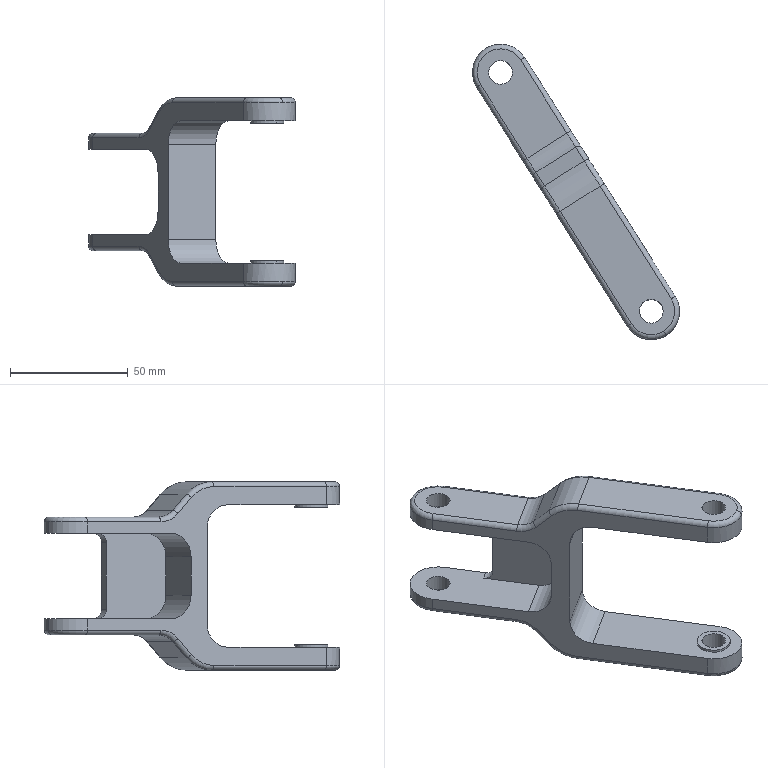Part | NX | features BREP 1 | 1 solid | 73 faces | box 88 x 125.509 x 80 mm | volume 73832 mm3 | cylinder 40 | plane 18 | torus 15 | commonest cylinder face diameters 4 x12 10.1 x8 20 x6 24 x6 14.1 x4 8 x2